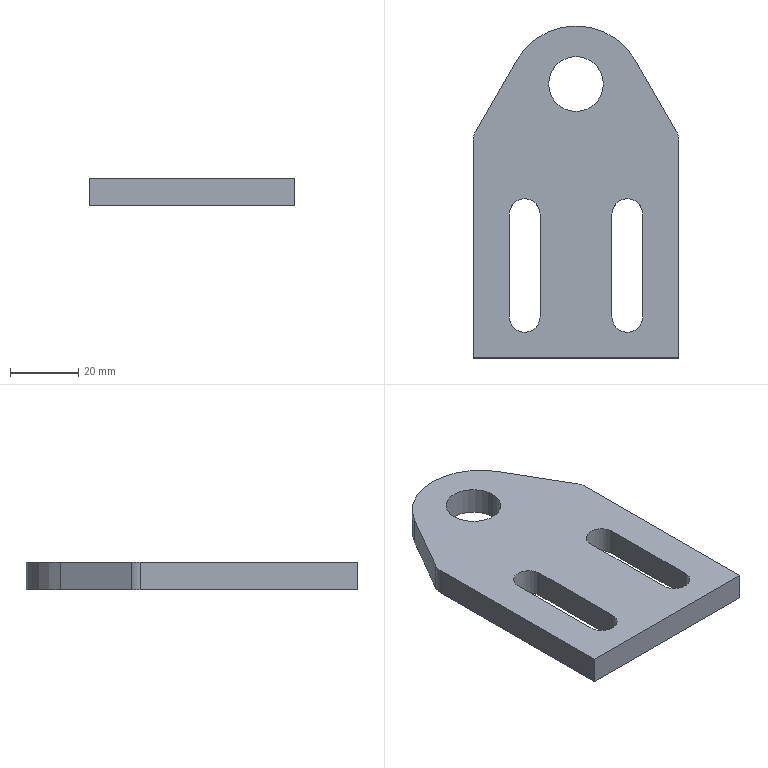Part | SolidWorks | features ICE 2, Extrusion 1, Fillet 1 | 1 solid | 20 faces | box 60 x 96.962 x 8 mm | volume 34530 mm3 | plane 11 | cylinder 9 | commonest cylinder face diameters 9 x4 10 x2 16 x2 40 x1
STEP:
#1=CARTESIAN_POINT('',(22.,80.,0.));
#2=VERTEX_POINT('',#1);
#3=CARTESIAN_POINT('',(38.,80.,0.));
#4=VERTEX_POINT('',#3);
#5=CARTESIAN_POINT('',(30.,80.,0.));
#6=DIRECTION('',(0.,0.,1.));
#7=DIRECTION('',(1.,0.,0.));
#8=AXIS2_PLACEMENT_3D('',#5,#6,#7);
#9=CIRCLE('',#8,8.);
#10=EDGE_CURVE('',#2,#4,#9,.T.);
#11=ORIENTED_EDGE('',*,*,#10,.F.);
#12=CARTESIAN_POINT('',(22.,80.,8.));
#13=VERTEX_POINT('',#12);
#14=CARTESIAN_POINT('',(22.,80.,0.));
#15=DIRECTION('',(0.,0.,1.));
#16=VECTOR('',#15,1000.);
#17=LINE('',#14,#16);
#18=EDGE_CURVE('',#2,#13,#17,.T.);
#19=ORIENTED_EDGE('',*,*,#18,.T.);
#20=CARTESIAN_POINT('',(38.,80.,8.));
#21=VERTEX_POINT('',#20);
#22=CARTESIAN_POINT('',(30.,80.,8.));
#23=DIRECTION('',(0.,0.,1.));
#24=DIRECTION('',(1.,0.,0.));
#25=AXIS2_PLACEMENT_3D('',#22,#23,#24);
#26=CIRCLE('',#25,8.);
#27=EDGE_CURVE('',#13,#21,#26,.T.);
#28=ORIENTED_EDGE('',*,*,#27,.T.);
#29=CARTESIAN_POINT('',(38.,80.,0.));
#30=DIRECTION('',(0.,0.,1.));
#31=VECTOR('',#30,1000.);
#32=LINE('',#29,#31);
#33=EDGE_CURVE('',#4,#21,#32,.T.);
#34=ORIENTED_EDGE('',*,*,#33,.F.);
#35=EDGE_LOOP('',(#11,#19,#28,#34));
#36=FACE_OUTER_BOUND('',#35,.T.);
#37=CARTESIAN_POINT('',(30.,80.,0.));
#38=DIRECTION('',(0.,0.,1.));
#39=DIRECTION('',(1.,0.,0.));
#40=AXIS2_PLACEMENT_3D('',#37,#38,#39);
#41=CYLINDRICAL_SURFACE('',#40,8.);
#42=ADVANCED_FACE('',(#36),#41,.F.);
#43=CARTESIAN_POINT('',(0.,0.,0.));
#44=VERTEX_POINT('',#43);
#45=CARTESIAN_POINT('',(60.,0.,0.));
#46=VERTEX_POINT('',#45);
#47=CARTESIAN_POINT('',(60.,0.,0.));
#48=DIRECTION('',(1.,0.,0.));
#49=VECTOR('',#48,1000.);
#50=LINE('',#47,#49);
#51=EDGE_CURVE('',#44,#46,#50,.T.);
#52=ORIENTED_EDGE('',*,*,#51,.T.);
#53=CARTESIAN_POINT('',(60.,0.,8.));
#54=VERTEX_POINT('',#53);
#55=CARTESIAN_POINT('',(60.,0.,8.));
#56=DIRECTION('',(0.,0.,-1.));
#57=VECTOR('',#56,1000.);
#58=LINE('',#55,#57);
#59=EDGE_CURVE('',#54,#46,#58,.T.);
#60=ORIENTED_EDGE('',*,*,#59,.F.);
#61=CARTESIAN_POINT('',(0.,0.,8.));
#62=VERTEX_POINT('',#61);
#63=CARTESIAN_POINT('',(60.,0.,8.));
#64=DIRECTION('',(1.,0.,0.));
#65=VECTOR('',#64,1000.);
#66=LINE('',#63,#65);
#67=EDGE_CURVE('',#62,#54,#66,.T.);
#68=ORIENTED_EDGE('',*,*,#67,.F.);
#69=CARTESIAN_POINT('',(0.,0.,8.));
#70=DIRECTION('',(0.,0.,-1.));
#71=VECTOR('',#70,1000.);
#72=LINE('',#69,#71);
#73=EDGE_CURVE('',#62,#44,#72,.T.);
#74=ORIENTED_EDGE('',*,*,#73,.T.);
#75=EDGE_LOOP('',(#52,#60,#68,#74));
#76=FACE_OUTER_BOUND('',#75,.T.);
#77=CARTESIAN_POINT('',(60.,0.,8.));
#78=DIRECTION('',(0.,1.,0.));
#79=DIRECTION('',(-1.,0.,0.));
#80=AXIS2_PLACEMENT_3D('',#77,#78,#79);
#81=PLANE('',#80);
#82=ADVANCED_FACE('',(#76),#81,.F.);
#83=CARTESIAN_POINT('',(60.,63.66,0.));
#84=VERTEX_POINT('',#83);
#85=CARTESIAN_POINT('',(60.,65.,0.));
#86=DIRECTION('',(0.,1.,0.));
#87=VECTOR('',#86,1000.);
#88=LINE('',#85,#87);
#89=EDGE_CURVE('',#46,#84,#88,.T.);
#90=ORIENTED_EDGE('',*,*,#89,.T.);
#91=CARTESIAN_POINT('',(60.,63.66,8.));
#92=VERTEX_POINT('',#91);
#93=CARTESIAN_POINT('',(60.,63.66,8.));
#94=DIRECTION('',(0.,0.,1.));
#95=VECTOR('',#94,1000.);
#96=LINE('',#93,#95);
#97=EDGE_CURVE('',#84,#92,#96,.T.);
#98=ORIENTED_EDGE('',*,*,#97,.T.);
#99=CARTESIAN_POINT('',(60.,65.,8.));
#100=DIRECTION('',(0.,1.,0.));
#101=VECTOR('',#100,1000.);
#102=LINE('',#99,#101);
#103=EDGE_CURVE('',#54,#92,#102,.T.);
#104=ORIENTED_EDGE('',*,*,#103,.F.);
#105=ORIENTED_EDGE('',*,*,#59,.T.);
#106=EDGE_LOOP('',(#90,#98,#104,#105));
#107=FACE_OUTER_BOUND('',#106,.T.);
#108=CARTESIAN_POINT('',(60.,65.,8.));
#109=DIRECTION('',(-1.,0.,0.));
#110=DIRECTION('',(0.,0.,1.));
#111=AXIS2_PLACEMENT_3D('',#108,#109,#110);
#112=PLANE('',#111);
#113=ADVANCED_FACE('',(#107),#112,.F.);
#114=CARTESIAN_POINT('',(59.33,66.16,8.));
#115=VERTEX_POINT('',#114);
#116=CARTESIAN_POINT('',(47.321,86.962,8.));
#117=VERTEX_POINT('',#116);
#118=CARTESIAN_POINT('',(47.321,86.962,8.));
#119=DIRECTION('',(-0.5,0.866,0.));
#120=VECTOR('',#119,1000.);
#121=LINE('',#118,#120);
#122=EDGE_CURVE('',#115,#117,#121,.T.);
#123=ORIENTED_EDGE('',*,*,#122,.F.);
#124=CARTESIAN_POINT('',(59.33,66.16,0.));
#125=VERTEX_POINT('',#124);
#126=CARTESIAN_POINT('',(59.33,66.16,8.));
#127=DIRECTION('',(0.,0.,-1.));
#128=VECTOR('',#127,1000.);
#129=LINE('',#126,#128);
#130=EDGE_CURVE('',#115,#125,#129,.T.);
#131=ORIENTED_EDGE('',*,*,#130,.T.);
#132=CARTESIAN_POINT('',(47.321,86.962,0.));
#133=VERTEX_POINT('',#132);
#134=CARTESIAN_POINT('',(47.321,86.962,0.));
#135=DIRECTION('',(-0.5,0.866,0.));
#136=VECTOR('',#135,1000.);
#137=LINE('',#134,#136);
#138=EDGE_CURVE('',#125,#133,#137,.T.);
#139=ORIENTED_EDGE('',*,*,#138,.T.);
#140=CARTESIAN_POINT('',(47.321,86.962,8.));
#141=DIRECTION('',(0.,0.,-1.));
#142=VECTOR('',#141,1000.);
#143=LINE('',#140,#142);
#144=EDGE_CURVE('',#117,#133,#143,.T.);
#145=ORIENTED_EDGE('',*,*,#144,.F.);
#146=EDGE_LOOP('',(#123,#131,#139,#145));
#147=FACE_OUTER_BOUND('',#146,.T.);
#148=CARTESIAN_POINT('',(47.321,86.962,8.));
#149=DIRECTION('',(-0.866,-0.5,0.));
#150=DIRECTION('',(0.5,-0.866,0.));
#151=AXIS2_PLACEMENT_3D('',#148,#149,#150);
#152=PLANE('',#151);
#153=ADVANCED_FACE('',(#147),#152,.F.);
#154=CARTESIAN_POINT('',(12.679,86.962,0.));
#155=VERTEX_POINT('',#154);
#156=CARTESIAN_POINT('',(30.,76.962,0.));
#157=DIRECTION('',(0.,0.,1.));
#158=DIRECTION('',(-1.,0.,0.));
#159=AXIS2_PLACEMENT_3D('',#156,#157,#158);
#160=CIRCLE('',#159,20.);
#161=EDGE_CURVE('',#133,#155,#160,.T.);
#162=ORIENTED_EDGE('',*,*,#161,.T.);
#163=CARTESIAN_POINT('',(12.679,86.962,8.));
#164=VERTEX_POINT('',#163);
#165=CARTESIAN_POINT('',(12.679,86.962,8.));
#166=DIRECTION('',(0.,0.,-1.));
#167=VECTOR('',#166,1000.);
#168=LINE('',#165,#167);
#169=EDGE_CURVE('',#164,#155,#168,.T.);
#170=ORIENTED_EDGE('',*,*,#169,.F.);
#171=CARTESIAN_POINT('',(30.,76.962,8.));
#172=DIRECTION('',(0.,0.,1.));
#173=DIRECTION('',(-1.,0.,0.));
#174=AXIS2_PLACEMENT_3D('',#171,#172,#173);
#175=CIRCLE('',#174,20.);
#176=EDGE_CURVE('',#117,#164,#175,.T.);
#177=ORIENTED_EDGE('',*,*,#176,.F.);
#178=ORIENTED_EDGE('',*,*,#144,.T.);
#179=EDGE_LOOP('',(#162,#170,#177,#178));
#180=FACE_OUTER_BOUND('',#179,.T.);
#181=CARTESIAN_POINT('',(30.,76.962,8.));
#182=DIRECTION('',(0.,0.,-1.));
#183=DIRECTION('',(-1.,0.,0.));
#184=AXIS2_PLACEMENT_3D('',#181,#182,#183);
#185=CYLINDRICAL_SURFACE('',#184,20.);
#186=ADVANCED_FACE('',(#180),#185,.T.);
#187=CARTESIAN_POINT('',(0.6699,66.16,0.));
#188=VERTEX_POINT('',#187);
#189=CARTESIAN_POINT('',(0.,65.,0.));
#190=DIRECTION('',(-0.5,-0.866,0.));
#191=VECTOR('',#190,1000.);
#192=LINE('',#189,#191);
#193=EDGE_CURVE('',#155,#188,#192,.T.);
#194=ORIENTED_EDGE('',*,*,#193,.T.);
#195=CARTESIAN_POINT('',(0.6699,66.16,8.));
#196=VERTEX_POINT('',#195);
#197=CARTESIAN_POINT('',(0.6699,66.16,8.));
#198=DIRECTION('',(0.,0.,1.));
#199=VECTOR('',#198,1000.);
#200=LINE('',#197,#199);
#201=EDGE_CURVE('',#188,#196,#200,.T.);
#202=ORIENTED_EDGE('',*,*,#201,.T.);
#203=CARTESIAN_POINT('',(0.,65.,8.));
#204=DIRECTION('',(-0.5,-0.866,0.));
#205=VECTOR('',#204,1000.);
#206=LINE('',#203,#205);
#207=EDGE_CURVE('',#164,#196,#206,.T.);
#208=ORIENTED_EDGE('',*,*,#207,.F.);
#209=ORIENTED_EDGE('',*,*,#169,.T.);
#210=EDGE_LOOP('',(#194,#202,#208,#209));
#211=FACE_OUTER_BOUND('',#210,.T.);
#212=CARTESIAN_POINT('',(0.,65.,8.));
#213=DIRECTION('',(0.866,-0.5,0.));
#214=DIRECTION('',(0.5,0.866,0.));
#215=AXIS2_PLACEMENT_3D('',#212,#213,#214);
#216=PLANE('',#215);
#217=ADVANCED_FACE('',(#211),#216,.F.);
#218=CARTESIAN_POINT('',(0.,63.66,8.));
#219=VERTEX_POINT('',#218);
#220=CARTESIAN_POINT('',(0.,0.,8.));
#221=DIRECTION('',(0.,-1.,0.));
#222=VECTOR('',#221,1000.);
#223=LINE('',#220,#222);
#224=EDGE_CURVE('',#219,#62,#223,.T.);
#225=ORIENTED_EDGE('',*,*,#224,.F.);
#226=CARTESIAN_POINT('',(0.,63.66,0.));
#227=VERTEX_POINT('',#226);
#228=CARTESIAN_POINT('',(0.,63.66,8.));
#229=DIRECTION('',(0.,0.,-1.));
#230=VECTOR('',#229,1000.);
#231=LINE('',#228,#230);
#232=EDGE_CURVE('',#219,#227,#231,.T.);
#233=ORIENTED_EDGE('',*,*,#232,.T.);
#234=CARTESIAN_POINT('',(0.,0.,0.));
#235=DIRECTION('',(0.,-1.,0.));
#236=VECTOR('',#235,1000.);
#237=LINE('',#234,#236);
#238=EDGE_CURVE('',#227,#44,#237,.T.);
#239=ORIENTED_EDGE('',*,*,#238,.T.);
#240=ORIENTED_EDGE('',*,*,#73,.F.);
#241=EDGE_LOOP('',(#225,#233,#239,#240));
#242=FACE_OUTER_BOUND('',#241,.T.);
#243=CARTESIAN_POINT('',(0.,0.,8.));
#244=DIRECTION('',(1.,0.,0.));
#245=DIRECTION('',(0.,0.,-1.));
#246=AXIS2_PLACEMENT_3D('',#243,#244,#245);
#247=PLANE('',#246);
#248=ADVANCED_FACE('',(#242),#247,.F.);
#249=CARTESIAN_POINT('',(19.5,12.,8.));
#250=VERTEX_POINT('',#249);
#251=CARTESIAN_POINT('',(19.5,42.,8.));
#252=VERTEX_POINT('',#251);
#253=CARTESIAN_POINT('',(19.5,12.,8.));
#254=DIRECTION('',(0.,1.,0.));
#255=VECTOR('',#254,1000.);
#256=LINE('',#253,#255);
#257=EDGE_CURVE('',#250,#252,#256,.T.);
#258=ORIENTED_EDGE('',*,*,#257,.F.);
#259=CARTESIAN_POINT('',(10.5,12.,8.));
#260=VERTEX_POINT('',#259);
#261=CARTESIAN_POINT('',(15.,12.,8.));
#262=DIRECTION('',(0.,0.,1.));
#263=DIRECTION('',(1.,0.,0.));
#264=AXIS2_PLACEMENT_3D('',#261,#262,#263);
#265=CIRCLE('',#264,4.5);
#266=EDGE_CURVE('',#260,#250,#265,.T.);
#267=ORIENTED_EDGE('',*,*,#266,.F.);
#268=CARTESIAN_POINT('',(10.5,42.,8.));
#269=VERTEX_POINT('',#268);
#270=CARTESIAN_POINT('',(10.5,12.,8.));
#271=DIRECTION('',(0.,-1.,0.));
#272=VECTOR('',#271,1000.);
#273=LINE('',#270,#272);
#274=EDGE_CURVE('',#269,#260,#273,.T.);
#275=ORIENTED_EDGE('',*,*,#274,.F.);
#276=CARTESIAN_POINT('',(15.,42.,8.));
#277=DIRECTION('',(0.,0.,1.));
#278=DIRECTION('',(1.,0.,0.));
#279=AXIS2_PLACEMENT_3D('',#276,#277,#278);
#280=CIRCLE('',#279,4.5);
#281=EDGE_CURVE('',#252,#269,#280,.T.);
#282=ORIENTED_EDGE('',*,*,#281,.F.);
#283=EDGE_LOOP('',(#258,#267,#275,#282));
#284=FACE_BOUND('',#283,.T.);
#285=CARTESIAN_POINT('',(49.5,12.,8.));
#286=VERTEX_POINT('',#285);
#287=CARTESIAN_POINT('',(49.5,42.,8.));
#288=VERTEX_POINT('',#287);
#289=CARTESIAN_POINT('',(49.5,12.,8.));
#290=DIRECTION('',(0.,1.,0.));
#291=VECTOR('',#290,1000.);
#292=LINE('',#289,#291);
#293=EDGE_CURVE('',#286,#288,#292,.T.);
#294=ORIENTED_EDGE('',*,*,#293,.F.);
#295=CARTESIAN_POINT('',(40.5,12.,8.));
#296=VERTEX_POINT('',#295);
#297=CARTESIAN_POINT('',(45.,12.,8.));
#298=DIRECTION('',(0.,0.,1.));
#299=DIRECTION('',(-1.,0.,0.));
#300=AXIS2_PLACEMENT_3D('',#297,#298,#299);
#301=CIRCLE('',#300,4.5);
#302=EDGE_CURVE('',#296,#286,#301,.T.);
#303=ORIENTED_EDGE('',*,*,#302,.F.);
#304=CARTESIAN_POINT('',(40.5,42.,8.));
#305=VERTEX_POINT('',#304);
#306=CARTESIAN_POINT('',(40.5,12.,8.));
#307=DIRECTION('',(0.,-1.,0.));
#308=VECTOR('',#307,1000.);
#309=LINE('',#306,#308);
#310=EDGE_CURVE('',#305,#296,#309,.T.);
#311=ORIENTED_EDGE('',*,*,#310,.F.);
#312=CARTESIAN_POINT('',(45.,42.,8.));
#313=DIRECTION('',(0.,0.,1.));
#314=DIRECTION('',(-1.,0.,0.));
#315=AXIS2_PLACEMENT_3D('',#312,#313,#314);
#316=CIRCLE('',#315,4.5);
#317=EDGE_CURVE('',#288,#305,#316,.T.);
#318=ORIENTED_EDGE('',*,*,#317,.F.);
#319=EDGE_LOOP('',(#294,#303,#311,#318));
#320=FACE_BOUND('',#319,.T.);
#321=CARTESIAN_POINT('',(30.,80.,8.));
#322=DIRECTION('',(0.,0.,1.));
#323=DIRECTION('',(1.,0.,0.));
#324=AXIS2_PLACEMENT_3D('',#321,#322,#323);
#325=CIRCLE('',#324,8.);
#326=EDGE_CURVE('',#21,#13,#325,.T.);
#327=ORIENTED_EDGE('',*,*,#326,.F.);
#328=ORIENTED_EDGE('',*,*,#27,.F.);
#329=EDGE_LOOP('',(#327,#328));
#330=FACE_BOUND('',#329,.T.);
#331=ORIENTED_EDGE('',*,*,#103,.T.);
#332=CARTESIAN_POINT('',(55.,63.66,8.));
#333=DIRECTION('',(0.,0.,1.));
#334=DIRECTION('',(-1.,0.,0.));
#335=AXIS2_PLACEMENT_3D('',#332,#333,#334);
#336=CIRCLE('',#335,5.);
#337=EDGE_CURVE('',#92,#115,#336,.T.);
#338=ORIENTED_EDGE('',*,*,#337,.T.);
#339=ORIENTED_EDGE('',*,*,#122,.T.);
#340=ORIENTED_EDGE('',*,*,#176,.T.);
#341=ORIENTED_EDGE('',*,*,#207,.T.);
#342=CARTESIAN_POINT('',(5.,63.66,8.));
#343=DIRECTION('',(0.,0.,1.));
#344=DIRECTION('',(-1.,0.,0.));
#345=AXIS2_PLACEMENT_3D('',#342,#343,#344);
#346=CIRCLE('',#345,5.);
#347=EDGE_CURVE('',#196,#219,#346,.T.);
#348=ORIENTED_EDGE('',*,*,#347,.T.);
#349=ORIENTED_EDGE('',*,*,#224,.T.);
#350=ORIENTED_EDGE('',*,*,#67,.T.);
#351=EDGE_LOOP('',(#331,#338,#339,#340,#341,#348,#349,#350));
#352=FACE_OUTER_BOUND('',#351,.T.);
#353=CARTESIAN_POINT('',(30.,76.962,8.));
#354=DIRECTION('',(0.,0.,-1.));
#355=DIRECTION('',(-1.,0.,0.));
#356=AXIS2_PLACEMENT_3D('',#353,#354,#355);
#357=PLANE('',#356);
#358=ADVANCED_FACE('',(#284,#320,#330,#352),#357,.F.);
#359=CARTESIAN_POINT('',(10.5,12.,0.));
#360=VERTEX_POINT('',#359);
#361=CARTESIAN_POINT('',(19.5,12.,0.));
#362=VERTEX_POINT('',#361);
#363=CARTESIAN_POINT('',(15.,12.,0.));
#364=DIRECTION('',(0.,0.,1.));
#365=DIRECTION('',(1.,0.,0.));
#366=AXIS2_PLACEMENT_3D('',#363,#364,#365);
#367=CIRCLE('',#366,4.5);
#368=EDGE_CURVE('',#360,#362,#367,.T.);
#369=ORIENTED_EDGE('',*,*,#368,.T.);
#370=CARTESIAN_POINT('',(19.5,42.,0.));
#371=VERTEX_POINT('',#370);
#372=CARTESIAN_POINT('',(19.5,12.,0.));
#373=DIRECTION('',(0.,1.,0.));
#374=VECTOR('',#373,1000.);
#375=LINE('',#372,#374);
#376=EDGE_CURVE('',#362,#371,#375,.T.);
#377=ORIENTED_EDGE('',*,*,#376,.T.);
#378=CARTESIAN_POINT('',(10.5,42.,0.));
#379=VERTEX_POINT('',#378);
#380=CARTESIAN_POINT('',(15.,42.,0.));
#381=DIRECTION('',(0.,0.,1.));
#382=DIRECTION('',(1.,0.,0.));
#383=AXIS2_PLACEMENT_3D('',#380,#381,#382);
#384=CIRCLE('',#383,4.5);
#385=EDGE_CURVE('',#371,#379,#384,.T.);
#386=ORIENTED_EDGE('',*,*,#385,.T.);
#387=CARTESIAN_POINT('',(10.5,12.,0.));
#388=DIRECTION('',(0.,-1.,0.));
#389=VECTOR('',#388,1000.);
#390=LINE('',#387,#389);
#391=EDGE_CURVE('',#379,#360,#390,.T.);
#392=ORIENTED_EDGE('',*,*,#391,.T.);
#393=EDGE_LOOP('',(#369,#377,#386,#392));
#394=FACE_BOUND('',#393,.T.);
#395=CARTESIAN_POINT('',(40.5,12.,0.));
#396=VERTEX_POINT('',#395);
#397=CARTESIAN_POINT('',(49.5,12.,0.));
#398=VERTEX_POINT('',#397);
#399=CARTESIAN_POINT('',(45.,12.,0.));
#400=DIRECTION('',(0.,0.,1.));
#401=DIRECTION('',(-1.,0.,0.));
#402=AXIS2_PLACEMENT_3D('',#399,#400,#401);
#403=CIRCLE('',#402,4.5);
#404=EDGE_CURVE('',#396,#398,#403,.T.);
#405=ORIENTED_EDGE('',*,*,#404,.T.);
#406=CARTESIAN_POINT('',(49.5,42.,0.));
#407=VERTEX_POINT('',#406);
#408=CARTESIAN_POINT('',(49.5,12.,0.));
#409=DIRECTION('',(0.,1.,0.));
#410=VECTOR('',#409,1000.);
#411=LINE('',#408,#410);
#412=EDGE_CURVE('',#398,#407,#411,.T.);
#413=ORIENTED_EDGE('',*,*,#412,.T.);
#414=CARTESIAN_POINT('',(40.5,42.,0.));
#415=VERTEX_POINT('',#414);
#416=CARTESIAN_POINT('',(45.,42.,0.));
#417=DIRECTION('',(0.,0.,1.));
#418=DIRECTION('',(-1.,0.,0.));
#419=AXIS2_PLACEMENT_3D('',#416,#417,#418);
#420=CIRCLE('',#419,4.5);
#421=EDGE_CURVE('',#407,#415,#420,.T.);
#422=ORIENTED_EDGE('',*,*,#421,.T.);
#423=CARTESIAN_POINT('',(40.5,12.,0.));
#424=DIRECTION('',(0.,-1.,0.));
#425=VECTOR('',#424,1000.);
#426=LINE('',#423,#425);
#427=EDGE_CURVE('',#415,#396,#426,.T.);
#428=ORIENTED_EDGE('',*,*,#427,.T.);
#429=EDGE_LOOP('',(#405,#413,#422,#428));
#430=FACE_BOUND('',#429,.T.);
#431=CARTESIAN_POINT('',(30.,80.,0.));
#432=DIRECTION('',(0.,0.,1.));
#433=DIRECTION('',(1.,0.,0.));
#434=AXIS2_PLACEMENT_3D('',#431,#432,#433);
#435=CIRCLE('',#434,8.);
#436=EDGE_CURVE('',#4,#2,#435,.T.);
#437=ORIENTED_EDGE('',*,*,#436,.T.);
#438=ORIENTED_EDGE('',*,*,#10,.T.);
#439=EDGE_LOOP('',(#437,#438));
#440=FACE_BOUND('',#439,.T.);
#441=ORIENTED_EDGE('',*,*,#138,.F.);
#442=CARTESIAN_POINT('',(55.,63.66,0.));
#443=DIRECTION('',(0.,0.,-1.));
#444=DIRECTION('',(-1.,0.,0.));
#445=AXIS2_PLACEMENT_3D('',#442,#443,#444);
#446=CIRCLE('',#445,5.);
#447=EDGE_CURVE('',#125,#84,#446,.T.);
#448=ORIENTED_EDGE('',*,*,#447,.T.);
#449=ORIENTED_EDGE('',*,*,#89,.F.);
#450=ORIENTED_EDGE('',*,*,#51,.F.);
#451=ORIENTED_EDGE('',*,*,#238,.F.);
#452=CARTESIAN_POINT('',(5.,63.66,0.));
#453=DIRECTION('',(0.,0.,-1.));
#454=DIRECTION('',(-1.,0.,0.));
#455=AXIS2_PLACEMENT_3D('',#452,#453,#454);
#456=CIRCLE('',#455,5.);
#457=EDGE_CURVE('',#227,#188,#456,.T.);
#458=ORIENTED_EDGE('',*,*,#457,.T.);
#459=ORIENTED_EDGE('',*,*,#193,.F.);
#460=ORIENTED_EDGE('',*,*,#161,.F.);
#461=EDGE_LOOP('',(#441,#448,#449,#450,#451,#458,#459,#460));
#462=FACE_OUTER_BOUND('',#461,.T.);
#463=CARTESIAN_POINT('',(30.,76.962,0.));
#464=DIRECTION('',(0.,0.,-1.));
#465=DIRECTION('',(-1.,0.,0.));
#466=AXIS2_PLACEMENT_3D('',#463,#464,#465);
#467=PLANE('',#466);
#468=ADVANCED_FACE('',(#394,#430,#440,#462),#467,.T.);
#469=ORIENTED_EDGE('',*,*,#18,.F.);
#470=ORIENTED_EDGE('',*,*,#436,.F.);
#471=ORIENTED_EDGE('',*,*,#33,.T.);
#472=ORIENTED_EDGE('',*,*,#326,.T.);
#473=EDGE_LOOP('',(#469,#470,#471,#472));
#474=FACE_OUTER_BOUND('',#473,.T.);
#475=CARTESIAN_POINT('',(30.,80.,0.));
#476=DIRECTION('',(0.,0.,1.));
#477=DIRECTION('',(1.,0.,0.));
#478=AXIS2_PLACEMENT_3D('',#475,#476,#477);
#479=CYLINDRICAL_SURFACE('',#478,8.);
#480=ADVANCED_FACE('',(#474),#479,.F.);
#481=ORIENTED_EDGE('',*,*,#302,.T.);
#482=CARTESIAN_POINT('',(49.5,12.,0.));
#483=DIRECTION('',(0.,0.,1.));
#484=VECTOR('',#483,1000.);
#485=LINE('',#482,#484);
#486=EDGE_CURVE('',#398,#286,#485,.T.);
#487=ORIENTED_EDGE('',*,*,#486,.F.);
#488=ORIENTED_EDGE('',*,*,#404,.F.);
#489=CARTESIAN_POINT('',(40.5,12.,0.));
#490=DIRECTION('',(0.,0.,1.));
#491=VECTOR('',#490,1000.);
#492=LINE('',#489,#491);
#493=EDGE_CURVE('',#396,#296,#492,.T.);
#494=ORIENTED_EDGE('',*,*,#493,.T.);
#495=EDGE_LOOP('',(#481,#487,#488,#494));
#496=FACE_OUTER_BOUND('',#495,.T.);
#497=CARTESIAN_POINT('',(45.,12.,0.));
#498=DIRECTION('',(0.,0.,1.));
#499=DIRECTION('',(1.,0.,0.));
#500=AXIS2_PLACEMENT_3D('',#497,#498,#499);
#501=CYLINDRICAL_SURFACE('',#500,4.5);
#502=ADVANCED_FACE('',(#496),#501,.F.);
#503=ORIENTED_EDGE('',*,*,#310,.T.);
#504=ORIENTED_EDGE('',*,*,#493,.F.);
#505=ORIENTED_EDGE('',*,*,#427,.F.);
#506=CARTESIAN_POINT('',(40.5,42.,0.));
#507=DIRECTION('',(0.,0.,1.));
#508=VECTOR('',#507,1000.);
#509=LINE('',#506,#508);
#510=EDGE_CURVE('',#415,#305,#509,.T.);
#511=ORIENTED_EDGE('',*,*,#510,.T.);
#512=EDGE_LOOP('',(#503,#504,#505,#511));
#513=FACE_OUTER_BOUND('',#512,.T.);
#514=CARTESIAN_POINT('',(40.5,12.,0.));
#515=DIRECTION('',(-1.,0.,0.));
#516=DIRECTION('',(0.,0.,1.));
#517=AXIS2_PLACEMENT_3D('',#514,#515,#516);
#518=PLANE('',#517);
#519=ADVANCED_FACE('',(#513),#518,.F.);
#520=ORIENTED_EDGE('',*,*,#317,.T.);
#521=ORIENTED_EDGE('',*,*,#510,.F.);
#522=ORIENTED_EDGE('',*,*,#421,.F.);
#523=CARTESIAN_POINT('',(49.5,42.,0.));
#524=DIRECTION('',(0.,0.,1.));
#525=VECTOR('',#524,1000.);
#526=LINE('',#523,#525);
#527=EDGE_CURVE('',#407,#288,#526,.T.);
#528=ORIENTED_EDGE('',*,*,#527,.T.);
#529=EDGE_LOOP('',(#520,#521,#522,#528));
#530=FACE_OUTER_BOUND('',#529,.T.);
#531=CARTESIAN_POINT('',(45.,42.,0.));
#532=DIRECTION('',(0.,0.,1.));
#533=DIRECTION('',(1.,0.,0.));
#534=AXIS2_PLACEMENT_3D('',#531,#532,#533);
#535=CYLINDRICAL_SURFACE('',#534,4.5);
#536=ADVANCED_FACE('',(#530),#535,.F.);
#537=ORIENTED_EDGE('',*,*,#293,.T.);
#538=ORIENTED_EDGE('',*,*,#527,.F.);
#539=ORIENTED_EDGE('',*,*,#412,.F.);
#540=ORIENTED_EDGE('',*,*,#486,.T.);
#541=EDGE_LOOP('',(#537,#538,#539,#540));
#542=FACE_OUTER_BOUND('',#541,.T.);
#543=CARTESIAN_POINT('',(49.5,12.,0.));
#544=DIRECTION('',(1.,0.,0.));
#545=DIRECTION('',(0.,0.,-1.));
#546=AXIS2_PLACEMENT_3D('',#543,#544,#545);
#547=PLANE('',#546);
#548=ADVANCED_FACE('',(#542),#547,.F.);
#549=ORIENTED_EDGE('',*,*,#266,.T.);
#550=CARTESIAN_POINT('',(19.5,12.,0.));
#551=DIRECTION('',(0.,0.,1.));
#552=VECTOR('',#551,1000.);
#553=LINE('',#550,#552);
#554=EDGE_CURVE('',#362,#250,#553,.T.);
#555=ORIENTED_EDGE('',*,*,#554,.F.);
#556=ORIENTED_EDGE('',*,*,#368,.F.);
#557=CARTESIAN_POINT('',(10.5,12.,0.));
#558=DIRECTION('',(0.,0.,1.));
#559=VECTOR('',#558,1000.);
#560=LINE('',#557,#559);
#561=EDGE_CURVE('',#360,#260,#560,.T.);
#562=ORIENTED_EDGE('',*,*,#561,.T.);
#563=EDGE_LOOP('',(#549,#555,#556,#562));
#564=FACE_OUTER_BOUND('',#563,.T.);
#565=CARTESIAN_POINT('',(15.,12.,0.));
#566=DIRECTION('',(0.,0.,1.));
#567=DIRECTION('',(1.,0.,0.));
#568=AXIS2_PLACEMENT_3D('',#565,#566,#567);
#569=CYLINDRICAL_SURFACE('',#568,4.5);
#570=ADVANCED_FACE('',(#564),#569,.F.);
#571=ORIENTED_EDGE('',*,*,#274,.T.);
#572=ORIENTED_EDGE('',*,*,#561,.F.);
#573=ORIENTED_EDGE('',*,*,#391,.F.);
#574=CARTESIAN_POINT('',(10.5,42.,0.));
#575=DIRECTION('',(0.,0.,1.));
#576=VECTOR('',#575,1000.);
#577=LINE('',#574,#576);
#578=EDGE_CURVE('',#379,#269,#577,.T.);
#579=ORIENTED_EDGE('',*,*,#578,.T.);
#580=EDGE_LOOP('',(#571,#572,#573,#579));
#581=FACE_OUTER_BOUND('',#580,.T.);
#582=CARTESIAN_POINT('',(10.5,12.,0.));
#583=DIRECTION('',(-1.,0.,0.));
#584=DIRECTION('',(0.,0.,1.));
#585=AXIS2_PLACEMENT_3D('',#582,#583,#584);
#586=PLANE('',#585);
#587=ADVANCED_FACE('',(#581),#586,.F.);
#588=ORIENTED_EDGE('',*,*,#281,.T.);
#589=ORIENTED_EDGE('',*,*,#578,.F.);
#590=ORIENTED_EDGE('',*,*,#385,.F.);
#591=CARTESIAN_POINT('',(19.5,42.,0.));
#592=DIRECTION('',(0.,0.,1.));
#593=VECTOR('',#592,1000.);
#594=LINE('',#591,#593);
#595=EDGE_CURVE('',#371,#252,#594,.T.);
#596=ORIENTED_EDGE('',*,*,#595,.T.);
#597=EDGE_LOOP('',(#588,#589,#590,#596));
#598=FACE_OUTER_BOUND('',#597,.T.);
#599=CARTESIAN_POINT('',(15.,42.,0.));
#600=DIRECTION('',(0.,0.,1.));
#601=DIRECTION('',(1.,0.,0.));
#602=AXIS2_PLACEMENT_3D('',#599,#600,#601);
#603=CYLINDRICAL_SURFACE('',#602,4.5);
#604=ADVANCED_FACE('',(#598),#603,.F.);
#605=ORIENTED_EDGE('',*,*,#257,.T.);
#606=ORIENTED_EDGE('',*,*,#595,.F.);
#607=ORIENTED_EDGE('',*,*,#376,.F.);
#608=ORIENTED_EDGE('',*,*,#554,.T.);
#609=EDGE_LOOP('',(#605,#606,#607,#608));
#610=FACE_OUTER_BOUND('',#609,.T.);
#611=CARTESIAN_POINT('',(19.5,12.,0.));
#612=DIRECTION('',(1.,0.,0.));
#613=DIRECTION('',(0.,0.,-1.));
#614=AXIS2_PLACEMENT_3D('',#611,#612,#613);
#615=PLANE('',#614);
#616=ADVANCED_FACE('',(#610),#615,.F.);
#617=ORIENTED_EDGE('',*,*,#337,.F.);
#618=ORIENTED_EDGE('',*,*,#97,.F.);
#619=ORIENTED_EDGE('',*,*,#447,.F.);
#620=ORIENTED_EDGE('',*,*,#130,.F.);
#621=EDGE_LOOP('',(#617,#618,#619,#620));
#622=FACE_OUTER_BOUND('',#621,.T.);
#623=CARTESIAN_POINT('',(55.,63.66,8.));
#624=DIRECTION('',(0.,0.,-1.));
#625=DIRECTION('',(-1.,0.,0.));
#626=AXIS2_PLACEMENT_3D('',#623,#624,#625);
#627=CYLINDRICAL_SURFACE('',#626,5.);
#628=ADVANCED_FACE('',(#622),#627,.T.);
#629=ORIENTED_EDGE('',*,*,#347,.F.);
#630=ORIENTED_EDGE('',*,*,#201,.F.);
#631=ORIENTED_EDGE('',*,*,#457,.F.);
#632=ORIENTED_EDGE('',*,*,#232,.F.);
#633=EDGE_LOOP('',(#629,#630,#631,#632));
#634=FACE_OUTER_BOUND('',#633,.T.);
#635=CARTESIAN_POINT('',(5.,63.66,8.));
#636=DIRECTION('',(0.,0.,-1.));
#637=DIRECTION('',(-1.,0.,0.));
#638=AXIS2_PLACEMENT_3D('',#635,#636,#637);
#639=CYLINDRICAL_SURFACE('',#638,5.);
#640=ADVANCED_FACE('',(#634),#639,.T.);
#641=CLOSED_SHELL('',(#42,#82,#113,#153,#186,#217,#248,#358,#468,#480,#502,#519,#536,#548,#570,#587,#604,#616,#628,#640));
#642=MANIFOLD_SOLID_BREP('',#641);
#643=CARTESIAN_POINT('',(0.,0.,0.));
#644=DIRECTION('',(0.,0.,1.));
#645=DIRECTION('',(1.,0.,0.));
#646=AXIS2_PLACEMENT_3D('',#643,#644,#645);
#647=(LENGTH_UNIT()NAMED_UNIT(*)SI_UNIT(.MILLI.,.METRE.));
#648=UNCERTAINTY_MEASURE_WITH_UNIT(LENGTH_MEASURE(0.00001),#647,'','');
#649=(NAMED_UNIT(*)PLANE_ANGLE_UNIT()SI_UNIT($,.RADIAN.));
#650=(NAMED_UNIT(*)SI_UNIT($,.STERADIAN.)SOLID_ANGLE_UNIT());
#651=(GEOMETRIC_REPRESENTATION_CONTEXT(3)GLOBAL_UNCERTAINTY_ASSIGNED_CONTEXT((#648))GLOBAL_UNIT_ASSIGNED_CONTEXT((#647,#649,#650))REPRESENTATION_CONTEXT('',''));
#652=ADVANCED_BREP_SHAPE_REPRESENTATION('',(#642,#646),#651);